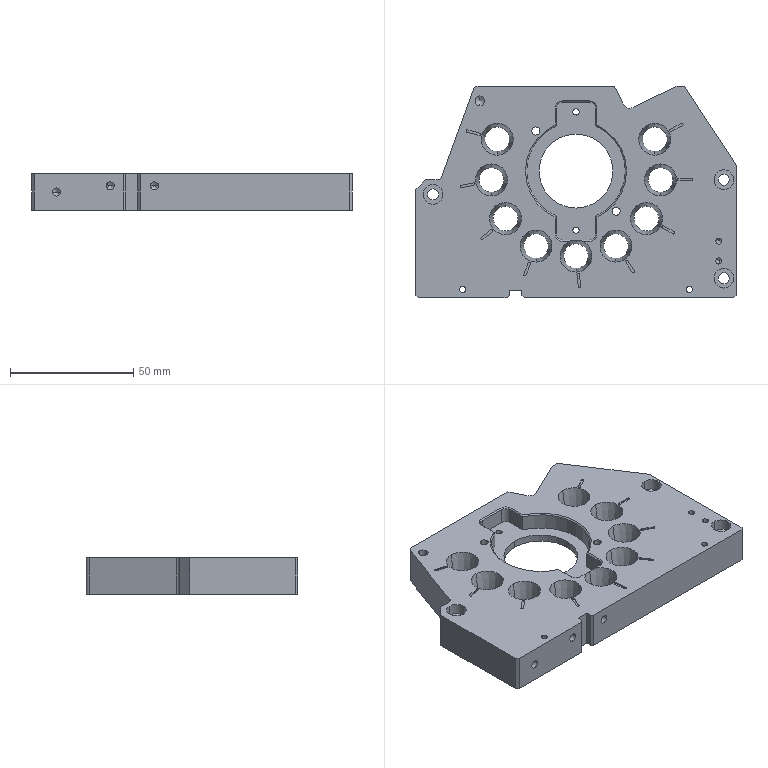NC program | NX | posted with a generic post | part box 130 x 86 x 15 mm
Lines 1 to 105 of 51277:
N10 G17 G21 G94 G90
(DRILLING , TOOL : ZXZ)
N12 T21 M6
N14 G54
N16 G17 G0 G90 X-39.5 Y46. B0. C0. S3500 M3
N18 G43 Z30. H21
N20 G94 G81 G98 Z-1. F250. R3.
N22 X-21.962 Y16.197
N24 X-10.792 Y28.602
N26 X-1. Y58.
N28 X4.894 Y34.311
N30 X21.424 Y31.988
N32 X37. Y39.
N34 X24.763 Y16.263
N36 X32.5 Y0.
N38 X8.5
N40 X-15.5
N42 X-21.962 Y-16.197
N44 X-7.763 Y-16.263
N46 X-10.792 Y-28.602
N48 X4.894 Y-34.311
N50 X21.424 Y-31.988
N52 X5. Y-60.
N54 X-20. Y-58.
N56 X-28.
N58 X-35. Y-60.
N60 X-39.5 Y-46.
N62 G80
N64 G0 X-39.5 Y-46. Z30.
N66 M5
(DRILLING_COPY_COPY , TOOL : 2.5ZT)
N68 T22 M6
N70 G54
N72 G17 G0 G90 X-39.5 Y46. B0. C0. S2000 M3
N74 G43 Z30. H22
N76 G94 G83 G98 Z-17.251 F150. Q2. R3.
N78 X-15.5 Y0.
N80 X32.5
N82 X-20. Y-58. Z-8.251
N84 X-28.
N86 X-39.5 Y-46. Z-17.251
N88 G80
N90 G0 X-39.5 Y-46. Z30.
N92 M5
(DRILLING_COPY_1 , TOOL : 3.3ZT)
N94 T13 M6
N96 G54
N98 G17 G0 G90 X-7.763 Y-16.263 B0. C0. S2000 M3
N100 G43 Z30. H13
N102 G94 G83 G98 Z-12.491 F150. Q2. R3.
N104 X24.763 Y16.263
N106 G80
N108 G0 X24.763 Y16.263 Z30.
N110 M5
(DRILLING_COPY_1_COPY , TOOL : 4.0ZT)
N112 T24 M6
N114 G54
N116 G17 G0 G90 X37. Y39. B0. C0. S2000 M3
N118 G43 Z30. H24
N120 G94 G83 G98 Z-6.202 F150. Q2. R3.
N122 G80
N124 G0 X37. Y39. Z30.
N126 M5
(DRILLING_COPY , TOOL : 4.5ZT)
N128 T12 M6
N130 G54
N132 G17 G0 G90 X-35. Y-60. B0. C0. S2000 M3
N134 G43 Z30. H12
N136 G94 G83 G98 Z-17.852 F150. Q2. R3.
N138 X5.
N140 X-1. Y58.
N142 G80
N144 G0 X-1. Y58. Z30.
N146 M5
(DRILLING_COPY_COPY_1 , TOOL : 10.ZT)
N148 T20 M6
N150 G54
N152 G17 G0 G90 X21.424 Y31.988 B0. C0. S2000 M3
N154 G43 Z30. H20
N156 G94 G83 G98 Z-19.504 F150. Q2. R3.
N158 X4.894 Y34.311
N160 X-10.792 Y28.602
N162 X-21.962 Y16.197
N164 X-26. Y0.
N166 X-21.962 Y-16.197
N168 X-10.792 Y-28.602
N170 X4.894 Y-34.311
N172 X21.424 Y-31.988
N174 G80
N176 G0 X21.424 Y-31.988 Z30.
N178 M5